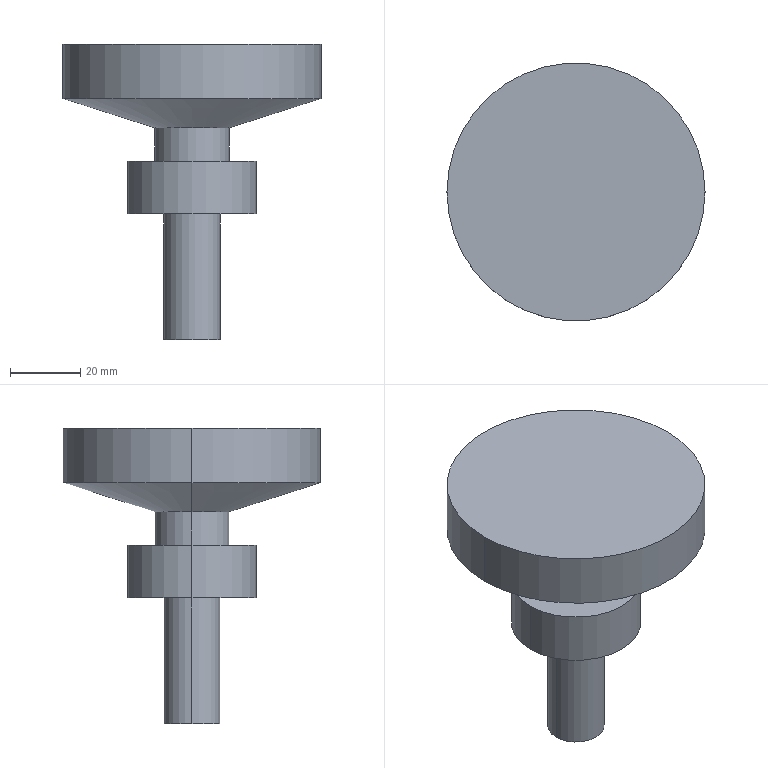Part | STEP file | M16 foot | 1 solid | 14 faces | box 73.343 x 73.343 x 84.032 mm | volume 107623 mm3 | cylinder 8 | plane 4 | cone 2 | commonest cylinder face diameters 16 x2 21.082 x2 36.671 x2 73.343 x2
STEP:
#1=CARTESIAN_POINT('',(0.,0.,0.));
#2=DIRECTION('',(0.,0.,1.));
#3=DIRECTION('',(1.,0.,0.));
#4=AXIS2_PLACEMENT_3D('',#1,#2,#3);
#5=CARTESIAN_POINT('',(-8.,0.,-48.252));
#6=VERTEX_POINT('',#5);
#7=CARTESIAN_POINT('',(8.,0.,-48.252));
#8=VERTEX_POINT('',#7);
#9=CARTESIAN_POINT('',(0.,0.,-48.252));
#10=DIRECTION('',(0.,0.,-1.));
#11=DIRECTION('',(-1.,0.,0.));
#12=AXIS2_PLACEMENT_3D('',#9,#10,#11);
#13=CIRCLE('',#12,8.);
#14=CARTESIAN_POINT('',(0.,0.,-84.032));
#15=DIRECTION('',(0.,0.,-1.));
#16=DIRECTION('',(-1.,0.,0.));
#17=AXIS2_PLACEMENT_3D('',#14,#15,#16);
#18=CYLINDRICAL_SURFACE('',#17,8.);
#19=CARTESIAN_POINT('',(0.,-35.78));
#20=DIRECTION('',(1.,0.));
#21=VECTOR('',#20,1.);
#22=LINE('',#19,#21);
#23=(GEOMETRIC_REPRESENTATION_CONTEXT(2)PARAMETRIC_REPRESENTATION_CONTEXT()REPRESENTATION_CONTEXT('',''));
#24=DEFINITIONAL_REPRESENTATION('',(#22),#23);
#25=PCURVE('',#18,#24);
#26=CARTESIAN_POINT('',(-18.336,0.,-48.252));
#27=DIRECTION('',(0.,0.,-1.));
#28=DIRECTION('',(-1.,0.,0.));
#29=AXIS2_PLACEMENT_3D('',#26,#27,#28);
#30=PLANE('',#29);
#31=CARTESIAN_POINT('',(-18.336,0.));
#32=DIRECTION('',(1.,0.));
#33=AXIS2_PLACEMENT_2D('',#31,#32);
#34=CIRCLE('',#33,8.);
#35=(GEOMETRIC_REPRESENTATION_CONTEXT(2)PARAMETRIC_REPRESENTATION_CONTEXT()REPRESENTATION_CONTEXT('',''));
#36=DEFINITIONAL_REPRESENTATION('',(#34),#35);
#37=PCURVE('',#30,#36);
#38=SURFACE_CURVE('',#13,(#25,#37),.PCURVE_S1.);
#39=EDGE_CURVE('',#6,#8,#38,.T.);
#40=ORIENTED_EDGE('',*,*,#39,.T.);
#41=CARTESIAN_POINT('',(8.,0.,-84.032));
#42=VERTEX_POINT('',#41);
#43=CARTESIAN_POINT('',(8.,0.,-84.032));
#44=DIRECTION('',(0.,0.,-1.));
#45=VECTOR('',#44,1.);
#46=LINE('',#43,#45);
#47=CARTESIAN_POINT('',(3.142,0.));
#48=DIRECTION('',(0.,1.));
#49=VECTOR('',#48,1.);
#50=LINE('',#47,#49);
#51=(GEOMETRIC_REPRESENTATION_CONTEXT(2)PARAMETRIC_REPRESENTATION_CONTEXT()REPRESENTATION_CONTEXT('',''));
#52=DEFINITIONAL_REPRESENTATION('',(#50),#51);
#53=PCURVE('',#18,#52);
#54=CARTESIAN_POINT('',(0.,0.,-84.032));
#55=DIRECTION('',(0.,0.,-1.));
#56=DIRECTION('',(-1.,0.,0.));
#57=AXIS2_PLACEMENT_3D('',#54,#55,#56);
#58=CYLINDRICAL_SURFACE('',#57,8.);
#59=CARTESIAN_POINT('',(3.142,0.));
#60=DIRECTION('',(0.,1.));
#61=VECTOR('',#60,1.);
#62=LINE('',#59,#61);
#63=(GEOMETRIC_REPRESENTATION_CONTEXT(2)PARAMETRIC_REPRESENTATION_CONTEXT()REPRESENTATION_CONTEXT('',''));
#64=DEFINITIONAL_REPRESENTATION('',(#62),#63);
#65=PCURVE('',#58,#64);
#66=SURFACE_CURVE('',#46,(#53,#65),.PCURVE_S1.);
#67=EDGE_CURVE('',#8,#42,#66,.T.);
#68=ORIENTED_EDGE('',*,*,#67,.T.);
#69=CARTESIAN_POINT('',(-8.,0.,-84.032));
#70=VERTEX_POINT('',#69);
#71=CARTESIAN_POINT('',(0.,0.,-84.032));
#72=DIRECTION('',(0.,0.,-1.));
#73=DIRECTION('',(-1.,0.,0.));
#74=AXIS2_PLACEMENT_3D('',#71,#72,#73);
#75=CIRCLE('',#74,8.);
#76=CARTESIAN_POINT('',(0.,0.));
#77=DIRECTION('',(1.,0.));
#78=VECTOR('',#77,1.);
#79=LINE('',#76,#78);
#80=(GEOMETRIC_REPRESENTATION_CONTEXT(2)PARAMETRIC_REPRESENTATION_CONTEXT()REPRESENTATION_CONTEXT('',''));
#81=DEFINITIONAL_REPRESENTATION('',(#79),#80);
#82=PCURVE('',#18,#81);
#83=CARTESIAN_POINT('',(-8.,0.,-84.032));
#84=DIRECTION('',(0.,0.,-1.));
#85=DIRECTION('',(-1.,0.,0.));
#86=AXIS2_PLACEMENT_3D('',#83,#84,#85);
#87=PLANE('',#86);
#88=CARTESIAN_POINT('',(-8.,0.));
#89=DIRECTION('',(1.,0.));
#90=AXIS2_PLACEMENT_2D('',#88,#89);
#91=CIRCLE('',#90,8.);
#92=(GEOMETRIC_REPRESENTATION_CONTEXT(2)PARAMETRIC_REPRESENTATION_CONTEXT()REPRESENTATION_CONTEXT('',''));
#93=DEFINITIONAL_REPRESENTATION('',(#91),#92);
#94=PCURVE('',#87,#93);
#95=SURFACE_CURVE('',#75,(#82,#94),.PCURVE_S1.);
#96=EDGE_CURVE('',#70,#42,#95,.T.);
#97=ORIENTED_EDGE('',*,*,#96,.F.);
#98=CARTESIAN_POINT('',(-8.,0.,-84.032));
#99=DIRECTION('',(0.,0.,-1.));
#100=VECTOR('',#99,1.);
#101=LINE('',#98,#100);
#102=CARTESIAN_POINT('',(0.,0.));
#103=DIRECTION('',(0.,1.));
#104=VECTOR('',#103,1.);
#105=LINE('',#102,#104);
#106=(GEOMETRIC_REPRESENTATION_CONTEXT(2)PARAMETRIC_REPRESENTATION_CONTEXT()REPRESENTATION_CONTEXT('',''));
#107=DEFINITIONAL_REPRESENTATION('',(#105),#106);
#108=PCURVE('',#18,#107);
#109=CARTESIAN_POINT('',(6.283,0.));
#110=DIRECTION('',(0.,1.));
#111=VECTOR('',#110,1.);
#112=LINE('',#109,#111);
#113=(GEOMETRIC_REPRESENTATION_CONTEXT(2)PARAMETRIC_REPRESENTATION_CONTEXT()REPRESENTATION_CONTEXT('',''));
#114=DEFINITIONAL_REPRESENTATION('',(#112),#113);
#115=PCURVE('',#58,#114);
#116=SURFACE_CURVE('',#101,(#108,#115),.PCURVE_S1.);
#117=EDGE_CURVE('',#6,#70,#116,.T.);
#118=ORIENTED_EDGE('',*,*,#117,.F.);
#119=EDGE_LOOP('',(#40,#68,#97,#118));
#120=FACE_BOUND('',#119,.T.);
#121=ADVANCED_FACE('',(#120),#18,.T.);
#122=CARTESIAN_POINT('',(-18.336,0.,-33.257));
#123=VERTEX_POINT('',#122);
#124=CARTESIAN_POINT('',(18.336,0.,-33.257));
#125=VERTEX_POINT('',#124);
#126=CARTESIAN_POINT('',(0.,0.,-33.257));
#127=DIRECTION('',(0.,0.,-1.));
#128=DIRECTION('',(-1.,0.,0.));
#129=AXIS2_PLACEMENT_3D('',#126,#127,#128);
#130=CIRCLE('',#129,18.336);
#131=CARTESIAN_POINT('',(0.,0.,-84.032));
#132=DIRECTION('',(0.,0.,-1.));
#133=DIRECTION('',(-1.,0.,0.));
#134=AXIS2_PLACEMENT_3D('',#131,#132,#133);
#135=CYLINDRICAL_SURFACE('',#134,18.336);
#136=CARTESIAN_POINT('',(0.,-50.776));
#137=DIRECTION('',(1.,0.));
#138=VECTOR('',#137,1.);
#139=LINE('',#136,#138);
#140=(GEOMETRIC_REPRESENTATION_CONTEXT(2)PARAMETRIC_REPRESENTATION_CONTEXT()REPRESENTATION_CONTEXT('',''));
#141=DEFINITIONAL_REPRESENTATION('',(#139),#140);
#142=PCURVE('',#135,#141);
#143=CARTESIAN_POINT('',(-10.541,0.,-33.257));
#144=DIRECTION('',(0.,0.,1.));
#145=DIRECTION('',(1.,0.,0.));
#146=AXIS2_PLACEMENT_3D('',#143,#144,#145);
#147=PLANE('',#146);
#148=CARTESIAN_POINT('',(-7.794,0.));
#149=CARTESIAN_POINT('',(-7.794,31.758));
#150=CARTESIAN_POINT('',(19.709,15.879));
#151=CARTESIAN_POINT('',(47.212,0.));
#152=CARTESIAN_POINT('',(19.709,-15.879));
#153=CARTESIAN_POINT('',(-7.794,-31.758));
#154=CARTESIAN_POINT('',(-7.794,0.));
#155=(BOUNDED_CURVE()B_SPLINE_CURVE(2,(#148,#149,#150,#151,#152,#153,#154),.UNSPECIFIED.,.T.,.F.)B_SPLINE_CURVE_WITH_KNOTS((1,2,2,2,2,1),(-2.094,0.,2.094,4.189,6.283,8.378),.UNSPECIFIED.)CURVE()GEOMETRIC_REPRESENTATION_ITEM()RATIONAL_B_SPLINE_CURVE((1.,0.5,1.,0.5,1.,0.5,1.))REPRESENTATION_ITEM(''));
#156=(GEOMETRIC_REPRESENTATION_CONTEXT(2)PARAMETRIC_REPRESENTATION_CONTEXT()REPRESENTATION_CONTEXT('',''));
#157=DEFINITIONAL_REPRESENTATION('',(#155),#156);
#158=PCURVE('',#147,#157);
#159=SURFACE_CURVE('',#130,(#142,#158),.PCURVE_S1.);
#160=EDGE_CURVE('',#123,#125,#159,.T.);
#161=ORIENTED_EDGE('',*,*,#160,.T.);
#162=CARTESIAN_POINT('',(18.336,0.,-48.252));
#163=VERTEX_POINT('',#162);
#164=CARTESIAN_POINT('',(18.336,0.,-84.032));
#165=DIRECTION('',(0.,0.,-1.));
#166=VECTOR('',#165,1.);
#167=LINE('',#164,#166);
#168=CARTESIAN_POINT('',(3.142,0.));
#169=DIRECTION('',(0.,1.));
#170=VECTOR('',#169,1.);
#171=LINE('',#168,#170);
#172=(GEOMETRIC_REPRESENTATION_CONTEXT(2)PARAMETRIC_REPRESENTATION_CONTEXT()REPRESENTATION_CONTEXT('',''));
#173=DEFINITIONAL_REPRESENTATION('',(#171),#172);
#174=PCURVE('',#135,#173);
#175=CARTESIAN_POINT('',(0.,0.,-84.032));
#176=DIRECTION('',(0.,0.,-1.));
#177=DIRECTION('',(-1.,0.,0.));
#178=AXIS2_PLACEMENT_3D('',#175,#176,#177);
#179=CYLINDRICAL_SURFACE('',#178,18.336);
#180=CARTESIAN_POINT('',(3.142,0.));
#181=DIRECTION('',(0.,1.));
#182=VECTOR('',#181,1.);
#183=LINE('',#180,#182);
#184=(GEOMETRIC_REPRESENTATION_CONTEXT(2)PARAMETRIC_REPRESENTATION_CONTEXT()REPRESENTATION_CONTEXT('',''));
#185=DEFINITIONAL_REPRESENTATION('',(#183),#184);
#186=PCURVE('',#179,#185);
#187=SURFACE_CURVE('',#167,(#174,#186),.PCURVE_S1.);
#188=EDGE_CURVE('',#125,#163,#187,.T.);
#189=ORIENTED_EDGE('',*,*,#188,.T.);
#190=CARTESIAN_POINT('',(-18.336,0.,-48.252));
#191=VERTEX_POINT('',#190);
#192=CARTESIAN_POINT('',(0.,0.,-48.252));
#193=DIRECTION('',(0.,0.,-1.));
#194=DIRECTION('',(-1.,0.,0.));
#195=AXIS2_PLACEMENT_3D('',#192,#193,#194);
#196=CIRCLE('',#195,18.336);
#197=CARTESIAN_POINT('',(0.,-35.78));
#198=DIRECTION('',(1.,0.));
#199=VECTOR('',#198,1.);
#200=LINE('',#197,#199);
#201=(GEOMETRIC_REPRESENTATION_CONTEXT(2)PARAMETRIC_REPRESENTATION_CONTEXT()REPRESENTATION_CONTEXT('',''));
#202=DEFINITIONAL_REPRESENTATION('',(#200),#201);
#203=PCURVE('',#135,#202);
#204=CARTESIAN_POINT('',(-18.336,0.));
#205=DIRECTION('',(1.,0.));
#206=AXIS2_PLACEMENT_2D('',#204,#205);
#207=CIRCLE('',#206,18.336);
#208=(GEOMETRIC_REPRESENTATION_CONTEXT(2)PARAMETRIC_REPRESENTATION_CONTEXT()REPRESENTATION_CONTEXT('',''));
#209=DEFINITIONAL_REPRESENTATION('',(#207),#208);
#210=PCURVE('',#30,#209);
#211=SURFACE_CURVE('',#196,(#203,#210),.PCURVE_S1.);
#212=EDGE_CURVE('',#191,#163,#211,.T.);
#213=ORIENTED_EDGE('',*,*,#212,.F.);
#214=CARTESIAN_POINT('',(-18.336,0.,-84.032));
#215=DIRECTION('',(0.,0.,-1.));
#216=VECTOR('',#215,1.);
#217=LINE('',#214,#216);
#218=CARTESIAN_POINT('',(0.,0.));
#219=DIRECTION('',(0.,1.));
#220=VECTOR('',#219,1.);
#221=LINE('',#218,#220);
#222=(GEOMETRIC_REPRESENTATION_CONTEXT(2)PARAMETRIC_REPRESENTATION_CONTEXT()REPRESENTATION_CONTEXT('',''));
#223=DEFINITIONAL_REPRESENTATION('',(#221),#222);
#224=PCURVE('',#135,#223);
#225=CARTESIAN_POINT('',(6.283,0.));
#226=DIRECTION('',(0.,1.));
#227=VECTOR('',#226,1.);
#228=LINE('',#225,#227);
#229=(GEOMETRIC_REPRESENTATION_CONTEXT(2)PARAMETRIC_REPRESENTATION_CONTEXT()REPRESENTATION_CONTEXT('',''));
#230=DEFINITIONAL_REPRESENTATION('',(#228),#229);
#231=PCURVE('',#179,#230);
#232=SURFACE_CURVE('',#217,(#224,#231),.PCURVE_S1.);
#233=EDGE_CURVE('',#123,#191,#232,.T.);
#234=ORIENTED_EDGE('',*,*,#233,.F.);
#235=EDGE_LOOP('',(#161,#189,#213,#234));
#236=FACE_BOUND('',#235,.T.);
#237=ADVANCED_FACE('',(#236),#135,.T.);
#238=CARTESIAN_POINT('',(-10.541,0.,-23.755));
#239=VERTEX_POINT('',#238);
#240=CARTESIAN_POINT('',(10.541,0.,-23.755));
#241=VERTEX_POINT('',#240);
#242=CARTESIAN_POINT('',(0.,0.,-23.755));
#243=DIRECTION('',(0.,0.,-1.));
#244=DIRECTION('',(-1.,0.,0.));
#245=AXIS2_PLACEMENT_3D('',#242,#243,#244);
#246=CIRCLE('',#245,10.541);
#247=CARTESIAN_POINT('',(0.,0.,-84.032));
#248=DIRECTION('',(0.,0.,-1.));
#249=DIRECTION('',(-1.,0.,0.));
#250=AXIS2_PLACEMENT_3D('',#247,#248,#249);
#251=CYLINDRICAL_SURFACE('',#250,10.541);
#252=CARTESIAN_POINT('',(0.,-60.277));
#253=DIRECTION('',(1.,0.));
#254=VECTOR('',#253,1.);
#255=LINE('',#252,#254);
#256=(GEOMETRIC_REPRESENTATION_CONTEXT(2)PARAMETRIC_REPRESENTATION_CONTEXT()REPRESENTATION_CONTEXT('',''));
#257=DEFINITIONAL_REPRESENTATION('',(#255),#256);
#258=PCURVE('',#251,#257);
#259=CARTESIAN_POINT('',(0.,0.,-23.755));
#260=DIRECTION('',(0.,0.,1.));
#261=DIRECTION('',(1.,0.,0.));
#262=AXIS2_PLACEMENT_3D('',#259,#260,#261);
#263=CONICAL_SURFACE('',#262,10.541,1.263);
#264=CARTESIAN_POINT('',(3.142,0.));
#265=DIRECTION('',(-1.,0.));
#266=VECTOR('',#265,1.);
#267=LINE('',#264,#266);
#268=(GEOMETRIC_REPRESENTATION_CONTEXT(2)PARAMETRIC_REPRESENTATION_CONTEXT()REPRESENTATION_CONTEXT('',''));
#269=DEFINITIONAL_REPRESENTATION('',(#267),#268);
#270=PCURVE('',#263,#269);
#271=SURFACE_CURVE('',#246,(#258,#270),.PCURVE_S1.);
#272=EDGE_CURVE('',#239,#241,#271,.T.);
#273=ORIENTED_EDGE('',*,*,#272,.T.);
#274=CARTESIAN_POINT('',(10.541,0.,-33.257));
#275=VERTEX_POINT('',#274);
#276=CARTESIAN_POINT('',(10.541,0.,-84.032));
#277=DIRECTION('',(0.,0.,-1.));
#278=VECTOR('',#277,1.);
#279=LINE('',#276,#278);
#280=CARTESIAN_POINT('',(3.142,0.));
#281=DIRECTION('',(0.,1.));
#282=VECTOR('',#281,1.);
#283=LINE('',#280,#282);
#284=(GEOMETRIC_REPRESENTATION_CONTEXT(2)PARAMETRIC_REPRESENTATION_CONTEXT()REPRESENTATION_CONTEXT('',''));
#285=DEFINITIONAL_REPRESENTATION('',(#283),#284);
#286=PCURVE('',#251,#285);
#287=CARTESIAN_POINT('',(0.,0.,-84.032));
#288=DIRECTION('',(0.,0.,-1.));
#289=DIRECTION('',(-1.,0.,0.));
#290=AXIS2_PLACEMENT_3D('',#287,#288,#289);
#291=CYLINDRICAL_SURFACE('',#290,10.541);
#292=CARTESIAN_POINT('',(3.142,0.));
#293=DIRECTION('',(0.,1.));
#294=VECTOR('',#293,1.);
#295=LINE('',#292,#294);
#296=(GEOMETRIC_REPRESENTATION_CONTEXT(2)PARAMETRIC_REPRESENTATION_CONTEXT()REPRESENTATION_CONTEXT('',''));
#297=DEFINITIONAL_REPRESENTATION('',(#295),#296);
#298=PCURVE('',#291,#297);
#299=SURFACE_CURVE('',#279,(#286,#298),.PCURVE_S1.);
#300=EDGE_CURVE('',#241,#275,#299,.T.);
#301=ORIENTED_EDGE('',*,*,#300,.T.);
#302=CARTESIAN_POINT('',(-10.541,0.,-33.257));
#303=VERTEX_POINT('',#302);
#304=CARTESIAN_POINT('',(0.,0.,-33.257));
#305=DIRECTION('',(0.,0.,-1.));
#306=DIRECTION('',(-1.,0.,0.));
#307=AXIS2_PLACEMENT_3D('',#304,#305,#306);
#308=CIRCLE('',#307,10.541);
#309=CARTESIAN_POINT('',(0.,-50.776));
#310=DIRECTION('',(1.,0.));
#311=VECTOR('',#310,1.);
#312=LINE('',#309,#311);
#313=(GEOMETRIC_REPRESENTATION_CONTEXT(2)PARAMETRIC_REPRESENTATION_CONTEXT()REPRESENTATION_CONTEXT('',''));
#314=DEFINITIONAL_REPRESENTATION('',(#312),#313);
#315=PCURVE('',#251,#314);
#316=CARTESIAN_POINT('',(0.,0.));
#317=CARTESIAN_POINT('',(0.,18.258));
#318=CARTESIAN_POINT('',(15.812,9.129));
#319=CARTESIAN_POINT('',(31.623,0.));
#320=CARTESIAN_POINT('',(15.812,-9.129));
#321=CARTESIAN_POINT('',(0.,-18.258));
#322=CARTESIAN_POINT('',(0.,0.));
#323=(BOUNDED_CURVE()B_SPLINE_CURVE(2,(#316,#317,#318,#319,#320,#321,#322),.UNSPECIFIED.,.T.,.F.)B_SPLINE_CURVE_WITH_KNOTS((1,2,2,2,2,1),(-2.094,0.,2.094,4.189,6.283,8.378),.UNSPECIFIED.)CURVE()GEOMETRIC_REPRESENTATION_ITEM()RATIONAL_B_SPLINE_CURVE((1.,0.5,1.,0.5,1.,0.5,1.))REPRESENTATION_ITEM(''));
#324=(GEOMETRIC_REPRESENTATION_CONTEXT(2)PARAMETRIC_REPRESENTATION_CONTEXT()REPRESENTATION_CONTEXT('',''));
#325=DEFINITIONAL_REPRESENTATION('',(#323),#324);
#326=PCURVE('',#147,#325);
#327=SURFACE_CURVE('',#308,(#315,#326),.PCURVE_S1.);
#328=EDGE_CURVE('',#303,#275,#327,.T.);
#329=ORIENTED_EDGE('',*,*,#328,.F.);
#330=CARTESIAN_POINT('',(-10.541,0.,-84.032));
#331=DIRECTION('',(0.,0.,-1.));
#332=VECTOR('',#331,1.);
#333=LINE('',#330,#332);
#334=CARTESIAN_POINT('',(0.,0.));
#335=DIRECTION('',(0.,1.));
#336=VECTOR('',#335,1.);
#337=LINE('',#334,#336);
#338=(GEOMETRIC_REPRESENTATION_CONTEXT(2)PARAMETRIC_REPRESENTATION_CONTEXT()REPRESENTATION_CONTEXT('',''));
#339=DEFINITIONAL_REPRESENTATION('',(#337),#338);
#340=PCURVE('',#251,#339);
#341=CARTESIAN_POINT('',(6.283,0.));
#342=DIRECTION('',(0.,1.));
#343=VECTOR('',#342,1.);
#344=LINE('',#341,#343);
#345=(GEOMETRIC_REPRESENTATION_CONTEXT(2)PARAMETRIC_REPRESENTATION_CONTEXT()REPRESENTATION_CONTEXT('',''));
#346=DEFINITIONAL_REPRESENTATION('',(#344),#345);
#347=PCURVE('',#291,#346);
#348=SURFACE_CURVE('',#333,(#340,#347),.PCURVE_S1.);
#349=EDGE_CURVE('',#239,#303,#348,.T.);
#350=ORIENTED_EDGE('',*,*,#349,.F.);
#351=EDGE_LOOP('',(#273,#301,#329,#350));
#352=FACE_BOUND('',#351,.T.);
#353=ADVANCED_FACE('',(#352),#251,.T.);
#354=ORIENTED_EDGE('',*,*,#272,.F.);
#355=CARTESIAN_POINT('',(-36.671,0.,-15.441));
#356=VERTEX_POINT('',#355);
#357=CARTESIAN_POINT('',(-10.541,0.,-23.755));
#358=DIRECTION('',(-0.9529,0.,0.3032));
#359=VECTOR('',#358,1.);
#360=LINE('',#357,#359);
#361=CARTESIAN_POINT('',(3.142,0.));
#362=DIRECTION('',(0.,1.));
#363=VECTOR('',#362,1.);
#364=LINE('',#361,#363);
#365=(GEOMETRIC_REPRESENTATION_CONTEXT(2)PARAMETRIC_REPRESENTATION_CONTEXT()REPRESENTATION_CONTEXT('',''));
#366=DEFINITIONAL_REPRESENTATION('',(#364),#365);
#367=PCURVE('',#263,#366);
#368=CARTESIAN_POINT('',(0.,0.,-23.755));
#369=DIRECTION('',(0.,0.,1.));
#370=DIRECTION('',(1.,0.,0.));
#371=AXIS2_PLACEMENT_3D('',#368,#369,#370);
#372=CONICAL_SURFACE('',#371,10.541,1.263);
#373=CARTESIAN_POINT('',(3.142,0.));
#374=DIRECTION('',(0.,1.));
#375=VECTOR('',#374,1.);
#376=LINE('',#373,#375);
#377=(GEOMETRIC_REPRESENTATION_CONTEXT(2)PARAMETRIC_REPRESENTATION_CONTEXT()REPRESENTATION_CONTEXT('',''));
#378=DEFINITIONAL_REPRESENTATION('',(#376),#377);
#379=PCURVE('',#372,#378);
#380=SURFACE_CURVE('',#360,(#367,#379),.PCURVE_S1.);
#381=EDGE_CURVE('',#239,#356,#380,.T.);
#382=ORIENTED_EDGE('',*,*,#381,.T.);
#383=CARTESIAN_POINT('',(36.671,0.,-15.441));
#384=VERTEX_POINT('',#383);
#385=CARTESIAN_POINT('',(0.,0.,-15.441));
#386=DIRECTION('',(0.,0.,-1.));
#387=DIRECTION('',(-1.,0.,0.));
#388=AXIS2_PLACEMENT_3D('',#385,#386,#387);
#389=CIRCLE('',#388,36.671);
#390=CARTESIAN_POINT('',(3.142,8.314));
#391=DIRECTION('',(-1.,0.));
#392=VECTOR('',#391,1.);
#393=LINE('',#390,#392);
#394=(GEOMETRIC_REPRESENTATION_CONTEXT(2)PARAMETRIC_REPRESENTATION_CONTEXT()REPRESENTATION_CONTEXT('',''));
#395=DEFINITIONAL_REPRESENTATION('',(#393),#394);
#396=PCURVE('',#263,#395);
#397=CARTESIAN_POINT('',(0.,0.,-84.032));
#398=DIRECTION('',(0.,0.,-1.));
#399=DIRECTION('',(-1.,0.,0.));
#400=AXIS2_PLACEMENT_3D('',#397,#398,#399);
#401=CYLINDRICAL_SURFACE('',#400,36.671);
#402=CARTESIAN_POINT('',(0.,-68.592));
#403=DIRECTION('',(1.,0.));
#404=VECTOR('',#403,1.);
#405=LINE('',#402,#404);
#406=(GEOMETRIC_REPRESENTATION_CONTEXT(2)PARAMETRIC_REPRESENTATION_CONTEXT()REPRESENTATION_CONTEXT('',''));
#407=DEFINITIONAL_REPRESENTATION('',(#405),#406);
#408=PCURVE('',#401,#407);
#409=SURFACE_CURVE('',#389,(#396,#408),.PCURVE_S1.);
#410=EDGE_CURVE('',#356,#384,#409,.T.);
#411=ORIENTED_EDGE('',*,*,#410,.T.);
#412=CARTESIAN_POINT('',(10.541,0.,-23.755));
#413=DIRECTION('',(0.9529,0.,0.3032));
#414=VECTOR('',#413,1.);
#415=LINE('',#412,#414);
#416=CARTESIAN_POINT('',(0.,0.));
#417=DIRECTION('',(0.,1.));
#418=VECTOR('',#417,1.);
#419=LINE('',#416,#418);
#420=(GEOMETRIC_REPRESENTATION_CONTEXT(2)PARAMETRIC_REPRESENTATION_CONTEXT()REPRESENTATION_CONTEXT('',''));
#421=DEFINITIONAL_REPRESENTATION('',(#419),#420);
#422=PCURVE('',#263,#421);
#423=CARTESIAN_POINT('',(6.283,0.));
#424=DIRECTION('',(0.,1.));
#425=VECTOR('',#424,1.);
#426=LINE('',#423,#425);
#427=(GEOMETRIC_REPRESENTATION_CONTEXT(2)PARAMETRIC_REPRESENTATION_CONTEXT()REPRESENTATION_CONTEXT('',''));
#428=DEFINITIONAL_REPRESENTATION('',(#426),#427);
#429=PCURVE('',#372,#428);
#430=SURFACE_CURVE('',#415,(#422,#429),.PCURVE_S1.);
#431=EDGE_CURVE('',#241,#384,#430,.T.);
#432=ORIENTED_EDGE('',*,*,#431,.F.);
#433=EDGE_LOOP('',(#354,#382,#411,#432));
#434=FACE_BOUND('',#433,.T.);
#435=ADVANCED_FACE('',(#434),#263,.T.);
#436=CARTESIAN_POINT('',(-36.671,0.,0.));
#437=VERTEX_POINT('',#436);
#438=CARTESIAN_POINT('',(36.671,0.,0.));
#439=VERTEX_POINT('',#438);
#440=CARTESIAN_POINT('',(0.,0.,0.));
#441=DIRECTION('',(0.,0.,-1.));
#442=DIRECTION('',(-1.,0.,0.));
#443=AXIS2_PLACEMENT_3D('',#440,#441,#442);
#444=CIRCLE('',#443,36.671);
#445=CARTESIAN_POINT('',(0.,-84.032));
#446=DIRECTION('',(1.,0.));
#447=VECTOR('',#446,1.);
#448=LINE('',#445,#447);
#449=(GEOMETRIC_REPRESENTATION_CONTEXT(2)PARAMETRIC_REPRESENTATION_CONTEXT()REPRESENTATION_CONTEXT('',''));
#450=DEFINITIONAL_REPRESENTATION('',(#448),#449);
#451=PCURVE('',#401,#450);
#452=CARTESIAN_POINT('',(0.,0.,0.));
#453=DIRECTION('',(0.,0.,1.));
#454=DIRECTION('',(1.,0.,0.));
#455=AXIS2_PLACEMENT_3D('',#452,#453,#454);
#456=PLANE('',#455);
#457=CARTESIAN_POINT('',(-36.671,0.));
#458=CARTESIAN_POINT('',(-36.671,63.516));
#459=CARTESIAN_POINT('',(18.336,31.758));
#460=CARTESIAN_POINT('',(73.343,0.));
#461=CARTESIAN_POINT('',(18.336,-31.758));
#462=CARTESIAN_POINT('',(-36.671,-63.516));
#463=CARTESIAN_POINT('',(-36.671,0.));
#464=(BOUNDED_CURVE()B_SPLINE_CURVE(2,(#457,#458,#459,#460,#461,#462,#463),.UNSPECIFIED.,.T.,.F.)B_SPLINE_CURVE_WITH_KNOTS((1,2,2,2,2,1),(-2.094,0.,2.094,4.189,6.283,8.378),.UNSPECIFIED.)CURVE()GEOMETRIC_REPRESENTATION_ITEM()RATIONAL_B_SPLINE_CURVE((1.,0.5,1.,0.5,1.,0.5,1.))REPRESENTATION_ITEM(''));
#465=(GEOMETRIC_REPRESENTATION_CONTEXT(2)PARAMETRIC_REPRESENTATION_CONTEXT()REPRESENTATION_CONTEXT('',''));
#466=DEFINITIONAL_REPRESENTATION('',(#464),#465);
#467=PCURVE('',#456,#466);
#468=SURFACE_CURVE('',#444,(#451,#467),.PCURVE_S1.);
#469=EDGE_CURVE('',#437,#439,#468,.T.);
#470=ORIENTED_EDGE('',*,*,#469,.T.);
#471=CARTESIAN_POINT('',(36.671,0.,-84.032));
#472=DIRECTION('',(0.,0.,-1.));
#473=VECTOR('',#472,1.);
#474=LINE('',#471,#473);
#475=CARTESIAN_POINT('',(3.142,0.));
#476=DIRECTION('',(0.,1.));
#477=VECTOR('',#476,1.);
#478=LINE('',#475,#477);
#479=(GEOMETRIC_REPRESENTATION_CONTEXT(2)PARAMETRIC_REPRESENTATION_CONTEXT()REPRESENTATION_CONTEXT('',''));
#480=DEFINITIONAL_REPRESENTATION('',(#478),#479);
#481=PCURVE('',#401,#480);
#482=CARTESIAN_POINT('',(0.,0.,-84.032));
#483=DIRECTION('',(0.,0.,-1.));
#484=DIRECTION('',(-1.,0.,0.));
#485=AXIS2_PLACEMENT_3D('',#482,#483,#484);
#486=CYLINDRICAL_SURFACE('',#485,36.671);
#487=CARTESIAN_POINT('',(3.142,0.));
#488=DIRECTION('',(0.,1.));
#489=VECTOR('',#488,1.);
#490=LINE('',#487,#489);
#491=(GEOMETRIC_REPRESENTATION_CONTEXT(2)PARAMETRIC_REPRESENTATION_CONTEXT()REPRESENTATION_CONTEXT('',''));
#492=DEFINITIONAL_REPRESENTATION('',(#490),#491);
#493=PCURVE('',#486,#492);
#494=SURFACE_CURVE('',#474,(#481,#493),.PCURVE_S1.);
#495=EDGE_CURVE('',#439,#384,#494,.T.);
#496=ORIENTED_EDGE('',*,*,#495,.T.);
#497=ORIENTED_EDGE('',*,*,#410,.F.);
#498=CARTESIAN_POINT('',(-36.671,0.,-84.032));
#499=DIRECTION('',(0.,0.,-1.));
#500=VECTOR('',#499,1.);
#501=LINE('',#498,#500);
#502=CARTESIAN_POINT('',(0.,0.));
#503=DIRECTION('',(0.,1.));
#504=VECTOR('',#503,1.);
#505=LINE('',#502,#504);
#506=(GEOMETRIC_REPRESENTATION_CONTEXT(2)PARAMETRIC_REPRESENTATION_CONTEXT()REPRESENTATION_CONTEXT('',''));
#507=DEFINITIONAL_REPRESENTATION('',(#505),#506);
#508=PCURVE('',#401,#507);
#509=CARTESIAN_POINT('',(6.283,0.));
#510=DIRECTION('',(0.,1.));
#511=VECTOR('',#510,1.);
#512=LINE('',#509,#511);
#513=(GEOMETRIC_REPRESENTATION_CONTEXT(2)PARAMETRIC_REPRESENTATION_CONTEXT()REPRESENTATION_CONTEXT('',''));
#514=DEFINITIONAL_REPRESENTATION('',(#512),#513);
#515=PCURVE('',#486,#514);
#516=SURFACE_CURVE('',#501,(#508,#515),.PCURVE_S1.);
#517=EDGE_CURVE('',#437,#356,#516,.T.);
#518=ORIENTED_EDGE('',*,*,#517,.F.);
#519=EDGE_LOOP('',(#470,#496,#497,#518));
#520=FACE_BOUND('',#519,.T.);
#521=ADVANCED_FACE('',(#520),#401,.T.);
#522=ORIENTED_EDGE('',*,*,#469,.F.);
#523=CARTESIAN_POINT('',(0.,0.,0.));
#524=DIRECTION('',(0.,0.,-1.));
#525=DIRECTION('',(-1.,0.,0.));
#526=AXIS2_PLACEMENT_3D('',#523,#524,#525);
#527=CIRCLE('',#526,36.671);
#528=CARTESIAN_POINT('',(-36.671,0.));
#529=CARTESIAN_POINT('',(-36.671,63.516));
#530=CARTESIAN_POINT('',(18.336,31.758));
#531=CARTESIAN_POINT('',(73.343,0.));
#532=CARTESIAN_POINT('',(18.336,-31.758));
#533=CARTESIAN_POINT('',(-36.671,-63.516));
#534=CARTESIAN_POINT('',(-36.671,0.));
#535=(BOUNDED_CURVE()B_SPLINE_CURVE(2,(#528,#529,#530,#531,#532,#533,#534),.UNSPECIFIED.,.T.,.F.)B_SPLINE_CURVE_WITH_KNOTS((1,2,2,2,2,1),(-2.094,0.,2.094,4.189,6.283,8.378),.UNSPECIFIED.)CURVE()GEOMETRIC_REPRESENTATION_ITEM()RATIONAL_B_SPLINE_CURVE((1.,0.5,1.,0.5,1.,0.5,1.))REPRESENTATION_ITEM(''));
#536=(GEOMETRIC_REPRESENTATION_CONTEXT(2)PARAMETRIC_REPRESENTATION_CONTEXT()REPRESENTATION_CONTEXT('',''));
#537=DEFINITIONAL_REPRESENTATION('',(#535),#536);
#538=PCURVE('',#456,#537);
#539=CARTESIAN_POINT('',(0.,-84.032));
#540=DIRECTION('',(1.,0.));
#541=VECTOR('',#540,1.);
#542=LINE('',#539,#541);
#543=(GEOMETRIC_REPRESENTATION_CONTEXT(2)PARAMETRIC_REPRESENTATION_CONTEXT()REPRESENTATION_CONTEXT('',''));
#544=DEFINITIONAL_REPRESENTATION('',(#542),#543);
#545=PCURVE('',#486,#544);
#546=SURFACE_CURVE('',#527,(#538,#545),.PCURVE_S1.);
#547=EDGE_CURVE('',#439,#437,#546,.T.);
#548=ORIENTED_EDGE('',*,*,#547,.F.);
#549=EDGE_LOOP('',(#522,#548));
#550=FACE_BOUND('',#549,.T.);
#551=ADVANCED_FACE('',(#550),#456,.T.);
#552=ORIENTED_EDGE('',*,*,#495,.F.);
#553=ORIENTED_EDGE('',*,*,#547,.T.);
#554=ORIENTED_EDGE('',*,*,#517,.T.);
#555=CARTESIAN_POINT('',(0.,0.,-15.441));
#556=DIRECTION('',(0.,0.,-1.));
#557=DIRECTION('',(-1.,0.,0.));
#558=AXIS2_PLACEMENT_3D('',#555,#556,#557);
#559=CIRCLE('',#558,36.671);
#560=CARTESIAN_POINT('',(0.,-68.592));
#561=DIRECTION('',(1.,0.));
#562=VECTOR('',#561,1.);
#563=LINE('',#560,#562);
#564=(GEOMETRIC_REPRESENTATION_CONTEXT(2)PARAMETRIC_REPRESENTATION_CONTEXT()REPRESENTATION_CONTEXT('',''));
#565=DEFINITIONAL_REPRESENTATION('',(#563),#564);
#566=PCURVE('',#486,#565);
#567=CARTESIAN_POINT('',(9.425,8.314));
#568=DIRECTION('',(-1.,0.));
#569=VECTOR('',#568,1.);
#570=LINE('',#567,#569);
#571=(GEOMETRIC_REPRESENTATION_CONTEXT(2)PARAMETRIC_REPRESENTATION_CONTEXT()REPRESENTATION_CONTEXT('',''));
#572=DEFINITIONAL_REPRESENTATION('',(#570),#571);
#573=PCURVE('',#372,#572);
#574=SURFACE_CURVE('',#559,(#566,#573),.PCURVE_S1.);
#575=EDGE_CURVE('',#384,#356,#574,.T.);
#576=ORIENTED_EDGE('',*,*,#575,.F.);
#577=EDGE_LOOP('',(#552,#553,#554,#576));
#578=FACE_BOUND('',#577,.T.);
#579=ADVANCED_FACE('',(#578),#486,.T.);
#580=ORIENTED_EDGE('',*,*,#381,.F.);
#581=CARTESIAN_POINT('',(0.,0.,-23.755));
#582=DIRECTION('',(0.,0.,-1.));
#583=DIRECTION('',(-1.,0.,0.));
#584=AXIS2_PLACEMENT_3D('',#581,#582,#583);
#585=CIRCLE('',#584,10.541);
#586=CARTESIAN_POINT('',(9.425,0.));
#587=DIRECTION('',(-1.,0.));
#588=VECTOR('',#587,1.);
#589=LINE('',#586,#588);
#590=(GEOMETRIC_REPRESENTATION_CONTEXT(2)PARAMETRIC_REPRESENTATION_CONTEXT()REPRESENTATION_CONTEXT('',''));
#591=DEFINITIONAL_REPRESENTATION('',(#589),#590);
#592=PCURVE('',#372,#591);
#593=CARTESIAN_POINT('',(0.,-60.277));
#594=DIRECTION('',(1.,0.));
#595=VECTOR('',#594,1.);
#596=LINE('',#593,#595);
#597=(GEOMETRIC_REPRESENTATION_CONTEXT(2)PARAMETRIC_REPRESENTATION_CONTEXT()REPRESENTATION_CONTEXT('',''));
#598=DEFINITIONAL_REPRESENTATION('',(#596),#597);
#599=PCURVE('',#291,#598);
#600=SURFACE_CURVE('',#585,(#592,#599),.PCURVE_S1.);
#601=EDGE_CURVE('',#241,#239,#600,.T.);
#602=ORIENTED_EDGE('',*,*,#601,.F.);
#603=ORIENTED_EDGE('',*,*,#431,.T.);
#604=ORIENTED_EDGE('',*,*,#575,.T.);
#605=EDGE_LOOP('',(#580,#602,#603,#604));
#606=FACE_BOUND('',#605,.T.);
#607=ADVANCED_FACE('',(#606),#372,.T.);
#608=ORIENTED_EDGE('',*,*,#300,.F.);
#609=ORIENTED_EDGE('',*,*,#601,.T.);
#610=ORIENTED_EDGE('',*,*,#349,.T.);
#611=CARTESIAN_POINT('',(0.,0.,-33.257));
#612=DIRECTION('',(0.,0.,-1.));
#613=DIRECTION('',(-1.,0.,0.));
#614=AXIS2_PLACEMENT_3D('',#611,#612,#613);
#615=CIRCLE('',#614,10.541);
#616=CARTESIAN_POINT('',(0.,-50.776));
#617=DIRECTION('',(1.,0.));
#618=VECTOR('',#617,1.);
#619=LINE('',#616,#618);
#620=(GEOMETRIC_REPRESENTATION_CONTEXT(2)PARAMETRIC_REPRESENTATION_CONTEXT()REPRESENTATION_CONTEXT('',''));
#621=DEFINITIONAL_REPRESENTATION('',(#619),#620);
#622=PCURVE('',#291,#621);
#623=CARTESIAN_POINT('',(0.,0.));
#624=CARTESIAN_POINT('',(0.,18.258));
#625=CARTESIAN_POINT('',(15.812,9.129));
#626=CARTESIAN_POINT('',(31.623,0.));
#627=CARTESIAN_POINT('',(15.812,-9.129));
#628=CARTESIAN_POINT('',(0.,-18.258));
#629=CARTESIAN_POINT('',(0.,0.));
#630=(BOUNDED_CURVE()B_SPLINE_CURVE(2,(#623,#624,#625,#626,#627,#628,#629),.UNSPECIFIED.,.T.,.F.)B_SPLINE_CURVE_WITH_KNOTS((1,2,2,2,2,1),(-2.094,0.,2.094,4.189,6.283,8.378),.UNSPECIFIED.)CURVE()GEOMETRIC_REPRESENTATION_ITEM()RATIONAL_B_SPLINE_CURVE((1.,0.5,1.,0.5,1.,0.5,1.))REPRESENTATION_ITEM(''));
#631=(GEOMETRIC_REPRESENTATION_CONTEXT(2)PARAMETRIC_REPRESENTATION_CONTEXT()REPRESENTATION_CONTEXT('',''));
#632=DEFINITIONAL_REPRESENTATION('',(#630),#631);
#633=PCURVE('',#147,#632);
#634=SURFACE_CURVE('',#615,(#622,#633),.PCURVE_S1.);
#635=EDGE_CURVE('',#275,#303,#634,.T.);
#636=ORIENTED_EDGE('',*,*,#635,.F.);
#637=EDGE_LOOP('',(#608,#609,#610,#636));
#638=FACE_BOUND('',#637,.T.);
#639=ADVANCED_FACE('',(#638),#291,.T.);
#640=ORIENTED_EDGE('',*,*,#328,.T.);
#641=ORIENTED_EDGE('',*,*,#635,.T.);
#642=EDGE_LOOP('',(#640,#641));
#643=FACE_BOUND('',#642,.T.);
#644=ORIENTED_EDGE('',*,*,#160,.F.);
#645=CARTESIAN_POINT('',(0.,0.,-33.257));
#646=DIRECTION('',(0.,0.,-1.));
#647=DIRECTION('',(-1.,0.,0.));
#648=AXIS2_PLACEMENT_3D('',#645,#646,#647);
#649=CIRCLE('',#648,18.336);
#650=CARTESIAN_POINT('',(-7.794,0.));
#651=CARTESIAN_POINT('',(-7.794,31.758));
#652=CARTESIAN_POINT('',(19.709,15.879));
#653=CARTESIAN_POINT('',(47.212,0.));
#654=CARTESIAN_POINT('',(19.709,-15.879));
#655=CARTESIAN_POINT('',(-7.794,-31.758));
#656=CARTESIAN_POINT('',(-7.794,0.));
#657=(BOUNDED_CURVE()B_SPLINE_CURVE(2,(#650,#651,#652,#653,#654,#655,#656),.UNSPECIFIED.,.T.,.F.)B_SPLINE_CURVE_WITH_KNOTS((1,2,2,2,2,1),(-2.094,0.,2.094,4.189,6.283,8.378),.UNSPECIFIED.)CURVE()GEOMETRIC_REPRESENTATION_ITEM()RATIONAL_B_SPLINE_CURVE((1.,0.5,1.,0.5,1.,0.5,1.))REPRESENTATION_ITEM(''));
#658=(GEOMETRIC_REPRESENTATION_CONTEXT(2)PARAMETRIC_REPRESENTATION_CONTEXT()REPRESENTATION_CONTEXT('',''));
#659=DEFINITIONAL_REPRESENTATION('',(#657),#658);
#660=PCURVE('',#147,#659);
#661=CARTESIAN_POINT('',(0.,-50.776));
#662=DIRECTION('',(1.,0.));
#663=VECTOR('',#662,1.);
#664=LINE('',#661,#663);
#665=(GEOMETRIC_REPRESENTATION_CONTEXT(2)PARAMETRIC_REPRESENTATION_CONTEXT()REPRESENTATION_CONTEXT('',''));
#666=DEFINITIONAL_REPRESENTATION('',(#664),#665);
#667=PCURVE('',#179,#666);
#668=SURFACE_CURVE('',#649,(#660,#667),.PCURVE_S1.);
#669=EDGE_CURVE('',#125,#123,#668,.T.);
#670=ORIENTED_EDGE('',*,*,#669,.F.);
#671=EDGE_LOOP('',(#644,#670));
#672=FACE_BOUND('',#671,.T.);
#673=ADVANCED_FACE('',(#643,#672),#147,.T.);
#674=ORIENTED_EDGE('',*,*,#188,.F.);
#675=ORIENTED_EDGE('',*,*,#669,.T.);
#676=ORIENTED_EDGE('',*,*,#233,.T.);
#677=CARTESIAN_POINT('',(0.,0.,-48.252));
#678=DIRECTION('',(0.,0.,-1.));
#679=DIRECTION('',(-1.,0.,0.));
#680=AXIS2_PLACEMENT_3D('',#677,#678,#679);
#681=CIRCLE('',#680,18.336);
#682=CARTESIAN_POINT('',(0.,-35.78));
#683=DIRECTION('',(1.,0.));
#684=VECTOR('',#683,1.);
#685=LINE('',#682,#684);
#686=(GEOMETRIC_REPRESENTATION_CONTEXT(2)PARAMETRIC_REPRESENTATION_CONTEXT()REPRESENTATION_CONTEXT('',''));
#687=DEFINITIONAL_REPRESENTATION('',(#685),#686);
#688=PCURVE('',#179,#687);
#689=CARTESIAN_POINT('',(-18.336,0.));
#690=DIRECTION('',(1.,0.));
#691=AXIS2_PLACEMENT_2D('',#689,#690);
#692=CIRCLE('',#691,18.336);
#693=(GEOMETRIC_REPRESENTATION_CONTEXT(2)PARAMETRIC_REPRESENTATION_CONTEXT()REPRESENTATION_CONTEXT('',''));
#694=DEFINITIONAL_REPRESENTATION('',(#692),#693);
#695=PCURVE('',#30,#694);
#696=SURFACE_CURVE('',#681,(#688,#695),.PCURVE_S1.);
#697=EDGE_CURVE('',#163,#191,#696,.T.);
#698=ORIENTED_EDGE('',*,*,#697,.F.);
#699=EDGE_LOOP('',(#674,#675,#676,#698));
#700=FACE_BOUND('',#699,.T.);
#701=ADVANCED_FACE('',(#700),#179,.T.);
#702=ORIENTED_EDGE('',*,*,#212,.T.);
#703=ORIENTED_EDGE('',*,*,#697,.T.);
#704=EDGE_LOOP('',(#702,#703));
#705=FACE_BOUND('',#704,.T.);
#706=ORIENTED_EDGE('',*,*,#39,.F.);
#707=CARTESIAN_POINT('',(0.,0.,-48.252));
#708=DIRECTION('',(0.,0.,-1.));
#709=DIRECTION('',(-1.,0.,0.));
#710=AXIS2_PLACEMENT_3D('',#707,#708,#709);
#711=CIRCLE('',#710,8.);
#712=CARTESIAN_POINT('',(-18.336,0.));
#713=DIRECTION('',(1.,0.));
#714=AXIS2_PLACEMENT_2D('',#712,#713);
#715=CIRCLE('',#714,8.);
#716=(GEOMETRIC_REPRESENTATION_CONTEXT(2)PARAMETRIC_REPRESENTATION_CONTEXT()REPRESENTATION_CONTEXT('',''));
#717=DEFINITIONAL_REPRESENTATION('',(#715),#716);
#718=PCURVE('',#30,#717);
#719=CARTESIAN_POINT('',(0.,-35.78));
#720=DIRECTION('',(1.,0.));
#721=VECTOR('',#720,1.);
#722=LINE('',#719,#721);
#723=(GEOMETRIC_REPRESENTATION_CONTEXT(2)PARAMETRIC_REPRESENTATION_CONTEXT()REPRESENTATION_CONTEXT('',''));
#724=DEFINITIONAL_REPRESENTATION('',(#722),#723);
#725=PCURVE('',#58,#724);
#726=SURFACE_CURVE('',#711,(#718,#725),.PCURVE_S1.);
#727=EDGE_CURVE('',#8,#6,#726,.T.);
#728=ORIENTED_EDGE('',*,*,#727,.F.);
#729=EDGE_LOOP('',(#706,#728));
#730=FACE_BOUND('',#729,.T.);
#731=ADVANCED_FACE('',(#705,#730),#30,.T.);
#732=ORIENTED_EDGE('',*,*,#67,.F.);
#733=ORIENTED_EDGE('',*,*,#727,.T.);
#734=ORIENTED_EDGE('',*,*,#117,.T.);
#735=CARTESIAN_POINT('',(0.,0.,-84.032));
#736=DIRECTION('',(0.,0.,-1.));
#737=DIRECTION('',(-1.,0.,0.));
#738=AXIS2_PLACEMENT_3D('',#735,#736,#737);
#739=CIRCLE('',#738,8.);
#740=CARTESIAN_POINT('',(0.,0.));
#741=DIRECTION('',(1.,0.));
#742=VECTOR('',#741,1.);
#743=LINE('',#740,#742);
#744=(GEOMETRIC_REPRESENTATION_CONTEXT(2)PARAMETRIC_REPRESENTATION_CONTEXT()REPRESENTATION_CONTEXT('',''));
#745=DEFINITIONAL_REPRESENTATION('',(#743),#744);
#746=PCURVE('',#58,#745);
#747=CARTESIAN_POINT('',(-8.,0.));
#748=DIRECTION('',(1.,0.));
#749=AXIS2_PLACEMENT_2D('',#747,#748);
#750=CIRCLE('',#749,8.);
#751=(GEOMETRIC_REPRESENTATION_CONTEXT(2)PARAMETRIC_REPRESENTATION_CONTEXT()REPRESENTATION_CONTEXT('',''));
#752=DEFINITIONAL_REPRESENTATION('',(#750),#751);
#753=PCURVE('',#87,#752);
#754=SURFACE_CURVE('',#739,(#746,#753),.PCURVE_S1.);
#755=EDGE_CURVE('',#42,#70,#754,.T.);
#756=ORIENTED_EDGE('',*,*,#755,.F.);
#757=EDGE_LOOP('',(#732,#733,#734,#756));
#758=FACE_BOUND('',#757,.T.);
#759=ADVANCED_FACE('',(#758),#58,.T.);
#760=ORIENTED_EDGE('',*,*,#96,.T.);
#761=ORIENTED_EDGE('',*,*,#755,.T.);
#762=EDGE_LOOP('',(#760,#761));
#763=FACE_BOUND('',#762,.T.);
#764=ADVANCED_FACE('',(#763),#87,.T.);
#765=CLOSED_SHELL('',(#121,#237,#353,#435,#521,#551,#579,#607,#639,#673,#701,#731,#759,#764));
#766=MANIFOLD_SOLID_BREP('',#765);
#767=(LENGTH_UNIT()NAMED_UNIT(*)SI_UNIT(.MILLI.,.METRE.));
#768=UNCERTAINTY_MEASURE_WITH_UNIT(LENGTH_MEASURE(0.0000001),#767,'','');
#769=(NAMED_UNIT(*)PLANE_ANGLE_UNIT()SI_UNIT($,.RADIAN.));
#770=(NAMED_UNIT(*)SI_UNIT($,.STERADIAN.)SOLID_ANGLE_UNIT());
#771=(GEOMETRIC_REPRESENTATION_CONTEXT(3)GLOBAL_UNCERTAINTY_ASSIGNED_CONTEXT((#768))GLOBAL_UNIT_ASSIGNED_CONTEXT((#767,#769,#770))REPRESENTATION_CONTEXT('',''));
#772=ADVANCED_BREP_SHAPE_REPRESENTATION('',(#4,#766),#771);